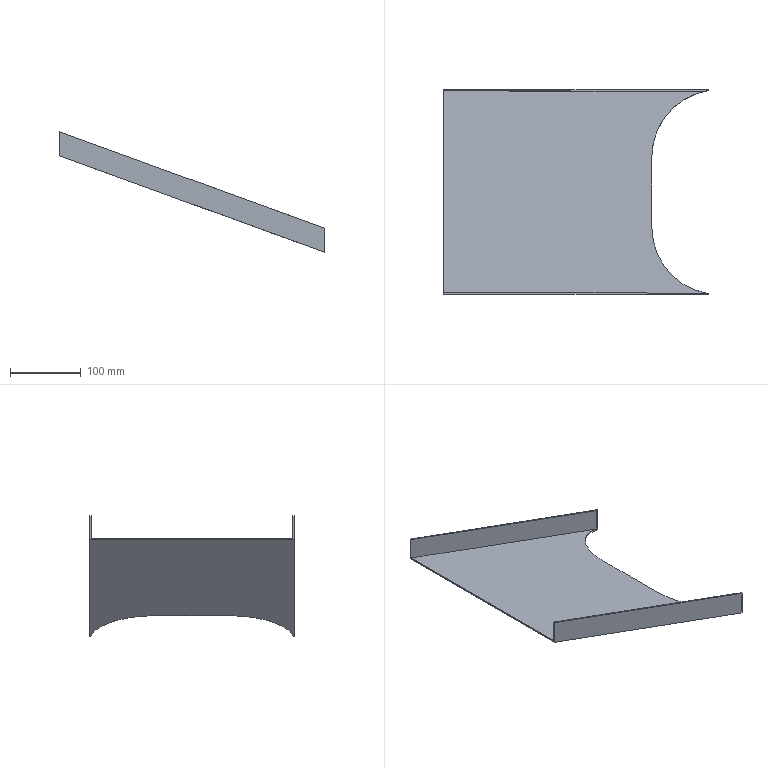Part | NX | features HB 2 | 1 solid | 14 faces | box 374.921 x 290 x 170.514 mm | volume 238011 mm3 | plane 12 | cylinder 2 | commonest cylinder face diameters 190 x2
STEP:
#1=CARTESIAN_POINT('',(630.,145.,-457.474));
#2=VERTEX_POINT('',#1);
#3=CARTESIAN_POINT('',(630.,143.808,-457.474));
#4=VERTEX_POINT('',#3);
#5=CARTESIAN_POINT('',(630.,203.921,-457.474));
#6=DIRECTION('',(0.,-1.,0.));
#7=VECTOR('',#6,1000.);
#8=LINE('',#5,#7);
#9=EDGE_CURVE('',#2,#4,#8,.T.);
#10=ORIENTED_EDGE('',*,*,#9,.T.);
#11=CARTESIAN_POINT('',(630.,143.808,-491.528));
#12=VERTEX_POINT('',#11);
#13=CARTESIAN_POINT('',(630.,143.808,-1480.5));
#14=DIRECTION('',(0.,0.,-1.));
#15=VECTOR('',#14,1000.);
#16=LINE('',#13,#15);
#17=EDGE_CURVE('',#4,#12,#16,.T.);
#18=ORIENTED_EDGE('',*,*,#17,.T.);
#19=CARTESIAN_POINT('',(630.,145.,-491.528));
#20=VERTEX_POINT('',#19);
#21=CARTESIAN_POINT('',(630.,98.921,-491.528));
#22=DIRECTION('',(0.,1.,0.));
#23=VECTOR('',#22,1000.);
#24=LINE('',#21,#23);
#25=EDGE_CURVE('',#12,#20,#24,.T.);
#26=ORIENTED_EDGE('',*,*,#25,.T.);
#27=CARTESIAN_POINT('',(630.,145.,-536.603));
#28=DIRECTION('',(0.,0.,1.));
#29=VECTOR('',#28,1000.);
#30=LINE('',#27,#29);
#31=EDGE_CURVE('',#20,#2,#30,.T.);
#32=ORIENTED_EDGE('',*,*,#31,.T.);
#33=EDGE_LOOP('',(#10,#18,#26,#32));
#34=FACE_BOUND('',#33,.T.);
#35=CARTESIAN_POINT('',(630.,0.,-678.5));
#36=DIRECTION('',(1.,0.,0.));
#37=DIRECTION('',(0.,0.,1.));
#38=AXIS2_PLACEMENT_3D('',#35,#36,#37);
#39=PLANE('',#38);
#40=ADVANCED_FACE('',(#34),#39,.T.);
#41=CARTESIAN_POINT('',(630.,-145.,-491.528));
#42=VERTEX_POINT('',#41);
#43=CARTESIAN_POINT('',(630.,-143.808,-491.528));
#44=VERTEX_POINT('',#43);
#45=CARTESIAN_POINT('',(630.,98.921,-491.528));
#46=DIRECTION('',(0.,1.,0.));
#47=VECTOR('',#46,1000.);
#48=LINE('',#45,#47);
#49=EDGE_CURVE('',#42,#44,#48,.T.);
#50=ORIENTED_EDGE('',*,*,#49,.T.);
#51=CARTESIAN_POINT('',(630.,-143.808,-457.474));
#52=VERTEX_POINT('',#51);
#53=CARTESIAN_POINT('',(630.,-143.808,-1480.5));
#54=DIRECTION('',(0.,0.,1.));
#55=VECTOR('',#54,1000.);
#56=LINE('',#53,#55);
#57=EDGE_CURVE('',#44,#52,#56,.T.);
#58=ORIENTED_EDGE('',*,*,#57,.T.);
#59=CARTESIAN_POINT('',(630.,-145.,-457.474));
#60=VERTEX_POINT('',#59);
#61=CARTESIAN_POINT('',(630.,-133.079,-457.474));
#62=DIRECTION('',(0.,-1.,0.));
#63=VECTOR('',#62,1000.);
#64=LINE('',#61,#63);
#65=EDGE_CURVE('',#52,#60,#64,.T.);
#66=ORIENTED_EDGE('',*,*,#65,.T.);
#67=CARTESIAN_POINT('',(630.,-145.,-2230.5));
#68=DIRECTION('',(0.,0.,-1.));
#69=VECTOR('',#68,1000.);
#70=LINE('',#67,#69);
#71=EDGE_CURVE('',#60,#42,#70,.T.);
#72=ORIENTED_EDGE('',*,*,#71,.T.);
#73=EDGE_LOOP('',(#50,#58,#66,#72));
#74=FACE_BOUND('',#73,.T.);
#75=CARTESIAN_POINT('',(630.,0.,-678.5));
#76=DIRECTION('',(1.,0.,0.));
#77=DIRECTION('',(0.,0.,1.));
#78=AXIS2_PLACEMENT_3D('',#75,#76,#77);
#79=PLANE('',#78);
#80=ADVANCED_FACE('',(#74),#79,.T.);
#81=CARTESIAN_POINT('',(625.609,-143.,-455.876));
#82=VERTEX_POINT('',#81);
#83=CARTESIAN_POINT('',(255.079,-143.,-321.014));
#84=VERTEX_POINT('',#83);
#85=CARTESIAN_POINT('',(1221.915,-143.,-672.914));
#86=DIRECTION('',(-0.9397,0.,0.342));
#87=VECTOR('',#86,1000.);
#88=LINE('',#85,#87);
#89=EDGE_CURVE('',#82,#84,#88,.T.);
#90=ORIENTED_EDGE('',*,*,#89,.F.);
#91=CARTESIAN_POINT('',(625.609,-143.,-487.801));
#92=VERTEX_POINT('',#91);
#93=CARTESIAN_POINT('',(625.609,-143.,-1480.5));
#94=DIRECTION('',(0.,0.,1.));
#95=VECTOR('',#94,1000.);
#96=LINE('',#93,#95);
#97=EDGE_CURVE('',#92,#82,#96,.T.);
#98=ORIENTED_EDGE('',*,*,#97,.F.);
#99=CARTESIAN_POINT('',(255.079,-143.,-352.939));
#100=VERTEX_POINT('',#99);
#101=CARTESIAN_POINT('',(1211.654,-143.,-701.104));
#102=DIRECTION('',(0.9397,0.,-0.342));
#103=VECTOR('',#102,1000.);
#104=LINE('',#101,#103);
#105=EDGE_CURVE('',#100,#92,#104,.T.);
#106=ORIENTED_EDGE('',*,*,#105,.F.);
#107=CARTESIAN_POINT('',(255.079,-143.,-160.));
#108=DIRECTION('',(0.,0.,-1.));
#109=VECTOR('',#108,1000.);
#110=LINE('',#107,#109);
#111=EDGE_CURVE('',#84,#100,#110,.T.);
#112=ORIENTED_EDGE('',*,*,#111,.F.);
#113=EDGE_LOOP('',(#90,#98,#106,#112));
#114=FACE_BOUND('',#113,.T.);
#115=CARTESIAN_POINT('',(655.,-143.,-2230.5));
#116=DIRECTION('',(0.,-1.,0.));
#117=DIRECTION('',(0.,0.,1.));
#118=AXIS2_PLACEMENT_3D('',#115,#116,#117);
#119=PLANE('',#118);
#120=ADVANCED_FACE('',(#114),#119,.F.);
#121=CARTESIAN_POINT('',(625.609,143.,-487.801));
#122=VERTEX_POINT('',#121);
#123=CARTESIAN_POINT('',(255.079,143.,-352.939));
#124=VERTEX_POINT('',#123);
#125=CARTESIAN_POINT('',(759.69,143.,-536.603));
#126=DIRECTION('',(-0.9397,0.,0.342));
#127=VECTOR('',#126,1000.);
#128=LINE('',#125,#127);
#129=EDGE_CURVE('',#122,#124,#128,.T.);
#130=ORIENTED_EDGE('',*,*,#129,.F.);
#131=CARTESIAN_POINT('',(625.609,143.,-455.876));
#132=VERTEX_POINT('',#131);
#133=CARTESIAN_POINT('',(625.609,143.,-1480.5));
#134=DIRECTION('',(0.,0.,1.));
#135=VECTOR('',#134,1000.);
#136=LINE('',#133,#135);
#137=EDGE_CURVE('',#122,#132,#136,.T.);
#138=ORIENTED_EDGE('',*,*,#137,.T.);
#139=CARTESIAN_POINT('',(255.079,143.,-321.014));
#140=VERTEX_POINT('',#139);
#141=CARTESIAN_POINT('',(769.951,143.,-508.412));
#142=DIRECTION('',(-0.9397,0.,0.342));
#143=VECTOR('',#142,1000.);
#144=LINE('',#141,#143);
#145=EDGE_CURVE('',#132,#140,#144,.T.);
#146=ORIENTED_EDGE('',*,*,#145,.T.);
#147=CARTESIAN_POINT('',(255.079,143.,-536.603));
#148=DIRECTION('',(0.,0.,1.));
#149=VECTOR('',#148,1000.);
#150=LINE('',#147,#149);
#151=EDGE_CURVE('',#124,#140,#150,.T.);
#152=ORIENTED_EDGE('',*,*,#151,.F.);
#153=EDGE_LOOP('',(#130,#138,#146,#152));
#154=FACE_BOUND('',#153,.T.);
#155=CARTESIAN_POINT('',(759.69,143.,-536.603));
#156=DIRECTION('',(0.,-1.,0.));
#157=DIRECTION('',(-0.08716,0.,0.9962));
#158=AXIS2_PLACEMENT_3D('',#155,#156,#157);
#159=PLANE('',#158);
#160=ADVANCED_FACE('',(#154),#159,.T.);
#161=CARTESIAN_POINT('',(645.,-50.,-462.934));
#162=DIRECTION('',(0.342,0.,0.9397));
#163=DIRECTION('',(-0.9397,0.,0.342));
#164=AXIS2_PLACEMENT_3D('',#161,#162,#163);
#165=ELLIPSE('',#164,101.097,95.);
#166=EDGE_CURVE('',#82,#52,#165,.T.);
#167=ORIENTED_EDGE('',*,*,#166,.F.);
#168=ORIENTED_EDGE('',*,*,#89,.T.);
#169=CARTESIAN_POINT('',(255.079,-145.,-321.014));
#170=VERTEX_POINT('',#169);
#171=CARTESIAN_POINT('',(255.079,-410.079,-321.014));
#172=DIRECTION('',(0.,-1.,0.));
#173=VECTOR('',#172,1000.);
#174=LINE('',#171,#173);
#175=EDGE_CURVE('',#84,#170,#174,.T.);
#176=ORIENTED_EDGE('',*,*,#175,.T.);
#177=CARTESIAN_POINT('',(1221.915,-145.,-672.914));
#178=DIRECTION('',(-0.9397,0.,0.342));
#179=VECTOR('',#178,1000.);
#180=LINE('',#177,#179);
#181=EDGE_CURVE('',#60,#170,#180,.T.);
#182=ORIENTED_EDGE('',*,*,#181,.F.);
#183=ORIENTED_EDGE('',*,*,#65,.F.);
#184=EDGE_LOOP('',(#167,#168,#176,#182,#183));
#185=FACE_BOUND('',#184,.T.);
#186=CARTESIAN_POINT('',(769.951,-133.079,-508.412));
#187=DIRECTION('',(-0.342,0.,-0.9397));
#188=DIRECTION('',(0.9397,0.,-0.342));
#189=AXIS2_PLACEMENT_3D('',#186,#187,#188);
#190=PLANE('',#189);
#191=ADVANCED_FACE('',(#185),#190,.F.);
#192=CARTESIAN_POINT('',(645.,50.,-462.934));
#193=DIRECTION('',(-0.342,0.,-0.9397));
#194=DIRECTION('',(-0.9397,0.,0.342));
#195=AXIS2_PLACEMENT_3D('',#192,#193,#194);
#196=ELLIPSE('',#195,101.097,95.);
#197=EDGE_CURVE('',#132,#4,#196,.T.);
#198=ORIENTED_EDGE('',*,*,#197,.T.);
#199=ORIENTED_EDGE('',*,*,#9,.F.);
#200=CARTESIAN_POINT('',(255.079,145.,-321.014));
#201=VERTEX_POINT('',#200);
#202=CARTESIAN_POINT('',(769.951,145.,-508.412));
#203=DIRECTION('',(-0.9397,0.,0.342));
#204=VECTOR('',#203,1000.);
#205=LINE('',#202,#204);
#206=EDGE_CURVE('',#2,#201,#205,.T.);
#207=ORIENTED_EDGE('',*,*,#206,.T.);
#208=CARTESIAN_POINT('',(255.079,-410.079,-321.014));
#209=DIRECTION('',(0.,-1.,0.));
#210=VECTOR('',#209,1000.);
#211=LINE('',#208,#210);
#212=EDGE_CURVE('',#201,#140,#211,.T.);
#213=ORIENTED_EDGE('',*,*,#212,.T.);
#214=ORIENTED_EDGE('',*,*,#145,.F.);
#215=EDGE_LOOP('',(#198,#199,#207,#213,#214));
#216=FACE_BOUND('',#215,.T.);
#217=CARTESIAN_POINT('',(769.951,203.921,-508.412));
#218=DIRECTION('',(-0.342,0.,-0.9397));
#219=DIRECTION('',(0.9397,0.,-0.342));
#220=AXIS2_PLACEMENT_3D('',#217,#218,#219);
#221=PLANE('',#220);
#222=ADVANCED_FACE('',(#216),#221,.F.);
#223=CARTESIAN_POINT('',(550.,50.,-460.282));
#224=VERTEX_POINT('',#223);
#225=CARTESIAN_POINT('',(550.,-50.,-460.282));
#226=VERTEX_POINT('',#225);
#227=CARTESIAN_POINT('',(550.,98.921,-460.282));
#228=DIRECTION('',(0.,-1.,0.));
#229=VECTOR('',#228,1000.);
#230=LINE('',#227,#229);
#231=EDGE_CURVE('',#224,#226,#230,.T.);
#232=ORIENTED_EDGE('',*,*,#231,.F.);
#233=CARTESIAN_POINT('',(645.,50.,-494.859));
#234=DIRECTION('',(0.342,0.,0.9397));
#235=DIRECTION('',(-0.9397,0.,0.342));
#236=AXIS2_PLACEMENT_3D('',#233,#234,#235);
#237=ELLIPSE('',#236,101.097,95.);
#238=EDGE_CURVE('',#122,#224,#237,.T.);
#239=ORIENTED_EDGE('',*,*,#238,.F.);
#240=ORIENTED_EDGE('',*,*,#129,.T.);
#241=CARTESIAN_POINT('',(255.079,-410.079,-352.939));
#242=DIRECTION('',(0.,1.,0.));
#243=VECTOR('',#242,1000.);
#244=LINE('',#241,#243);
#245=EDGE_CURVE('',#100,#124,#244,.T.);
#246=ORIENTED_EDGE('',*,*,#245,.F.);
#247=ORIENTED_EDGE('',*,*,#105,.T.);
#248=CARTESIAN_POINT('',(645.,-50.,-494.859));
#249=DIRECTION('',(0.342,0.,0.9397));
#250=DIRECTION('',(-0.9397,0.,0.342));
#251=AXIS2_PLACEMENT_3D('',#248,#249,#250);
#252=ELLIPSE('',#251,101.097,95.);
#253=EDGE_CURVE('',#226,#92,#252,.T.);
#254=ORIENTED_EDGE('',*,*,#253,.F.);
#255=EDGE_LOOP('',(#232,#239,#240,#246,#247,#254));
#256=FACE_BOUND('',#255,.T.);
#257=CARTESIAN_POINT('',(759.69,98.921,-536.603));
#258=DIRECTION('',(0.342,0.,0.9397));
#259=DIRECTION('',(0.,-1.,0.));
#260=AXIS2_PLACEMENT_3D('',#257,#258,#259);
#261=PLANE('',#260);
#262=ADVANCED_FACE('',(#256),#261,.T.);
#263=CARTESIAN_POINT('',(550.,50.,-462.41));
#264=VERTEX_POINT('',#263);
#265=CARTESIAN_POINT('',(645.,50.,-496.987));
#266=DIRECTION('',(-0.342,0.,-0.9397));
#267=DIRECTION('',(-0.9397,0.,0.342));
#268=AXIS2_PLACEMENT_3D('',#265,#266,#267);
#269=ELLIPSE('',#268,101.097,95.);
#270=EDGE_CURVE('',#264,#12,#269,.T.);
#271=ORIENTED_EDGE('',*,*,#270,.F.);
#272=CARTESIAN_POINT('',(550.,-50.,-462.41));
#273=VERTEX_POINT('',#272);
#274=CARTESIAN_POINT('',(550.,98.921,-462.41));
#275=DIRECTION('',(0.,1.,0.));
#276=VECTOR('',#275,1000.);
#277=LINE('',#274,#276);
#278=EDGE_CURVE('',#273,#264,#277,.T.);
#279=ORIENTED_EDGE('',*,*,#278,.F.);
#280=CARTESIAN_POINT('',(645.,-50.,-496.987));
#281=DIRECTION('',(0.342,0.,0.9397));
#282=DIRECTION('',(-0.9397,0.,0.342));
#283=AXIS2_PLACEMENT_3D('',#280,#281,#282);
#284=ELLIPSE('',#283,101.097,95.);
#285=EDGE_CURVE('',#273,#44,#284,.T.);
#286=ORIENTED_EDGE('',*,*,#285,.T.);
#287=ORIENTED_EDGE('',*,*,#49,.F.);
#288=CARTESIAN_POINT('',(255.079,-145.,-355.068));
#289=VERTEX_POINT('',#288);
#290=CARTESIAN_POINT('',(759.006,-145.,-538.482));
#291=DIRECTION('',(-0.9397,0.,0.342));
#292=VECTOR('',#291,1000.);
#293=LINE('',#290,#292);
#294=EDGE_CURVE('',#42,#289,#293,.T.);
#295=ORIENTED_EDGE('',*,*,#294,.T.);
#296=CARTESIAN_POINT('',(255.079,145.,-355.068));
#297=VERTEX_POINT('',#296);
#298=CARTESIAN_POINT('',(255.079,-410.079,-355.068));
#299=DIRECTION('',(0.,1.,0.));
#300=VECTOR('',#299,1000.);
#301=LINE('',#298,#300);
#302=EDGE_CURVE('',#289,#297,#301,.T.);
#303=ORIENTED_EDGE('',*,*,#302,.T.);
#304=CARTESIAN_POINT('',(759.006,145.,-538.482));
#305=DIRECTION('',(0.9397,0.,-0.342));
#306=VECTOR('',#305,1000.);
#307=LINE('',#304,#306);
#308=EDGE_CURVE('',#297,#20,#307,.T.);
#309=ORIENTED_EDGE('',*,*,#308,.T.);
#310=ORIENTED_EDGE('',*,*,#25,.F.);
#311=EDGE_LOOP('',(#271,#279,#286,#287,#295,#303,#309,#310));
#312=FACE_BOUND('',#311,.T.);
#313=CARTESIAN_POINT('',(759.006,98.921,-538.482));
#314=DIRECTION('',(0.342,0.,0.9397));
#315=DIRECTION('',(0.,-1.,0.));
#316=AXIS2_PLACEMENT_3D('',#313,#314,#315);
#317=PLANE('',#316);
#318=ADVANCED_FACE('',(#312),#317,.F.);
#319=ORIENTED_EDGE('',*,*,#31,.F.);
#320=ORIENTED_EDGE('',*,*,#308,.F.);
#321=CARTESIAN_POINT('',(255.079,145.,-536.603));
#322=DIRECTION('',(0.,0.,1.));
#323=VECTOR('',#322,1000.);
#324=LINE('',#321,#323);
#325=EDGE_CURVE('',#297,#201,#324,.T.);
#326=ORIENTED_EDGE('',*,*,#325,.T.);
#327=ORIENTED_EDGE('',*,*,#206,.F.);
#328=EDGE_LOOP('',(#319,#320,#326,#327));
#329=FACE_BOUND('',#328,.T.);
#330=CARTESIAN_POINT('',(759.69,145.,-536.603));
#331=DIRECTION('',(0.,-1.,0.));
#332=DIRECTION('',(0.08716,0.,-0.9962));
#333=AXIS2_PLACEMENT_3D('',#330,#331,#332);
#334=PLANE('',#333);
#335=ADVANCED_FACE('',(#329),#334,.F.);
#336=ORIENTED_EDGE('',*,*,#71,.F.);
#337=ORIENTED_EDGE('',*,*,#181,.T.);
#338=CARTESIAN_POINT('',(255.079,-145.,-160.));
#339=DIRECTION('',(0.,0.,-1.));
#340=VECTOR('',#339,1000.);
#341=LINE('',#338,#340);
#342=EDGE_CURVE('',#170,#289,#341,.T.);
#343=ORIENTED_EDGE('',*,*,#342,.T.);
#344=ORIENTED_EDGE('',*,*,#294,.F.);
#345=EDGE_LOOP('',(#336,#337,#343,#344));
#346=FACE_BOUND('',#345,.T.);
#347=CARTESIAN_POINT('',(655.,-145.,-2230.5));
#348=DIRECTION('',(0.,-1.,0.));
#349=DIRECTION('',(0.,0.,1.));
#350=AXIS2_PLACEMENT_3D('',#347,#348,#349);
#351=PLANE('',#350);
#352=ADVANCED_FACE('',(#346),#351,.T.);
#353=ORIENTED_EDGE('',*,*,#302,.F.);
#354=ORIENTED_EDGE('',*,*,#342,.F.);
#355=ORIENTED_EDGE('',*,*,#175,.F.);
#356=ORIENTED_EDGE('',*,*,#111,.T.);
#357=ORIENTED_EDGE('',*,*,#245,.T.);
#358=ORIENTED_EDGE('',*,*,#151,.T.);
#359=ORIENTED_EDGE('',*,*,#212,.F.);
#360=ORIENTED_EDGE('',*,*,#325,.F.);
#361=EDGE_LOOP('',(#353,#354,#355,#356,#357,#358,#359,#360));
#362=FACE_BOUND('',#361,.T.);
#363=CARTESIAN_POINT('',(255.079,-410.079,-160.));
#364=DIRECTION('',(-1.,0.,0.));
#365=DIRECTION('',(0.,0.,-1.));
#366=AXIS2_PLACEMENT_3D('',#363,#364,#365);
#367=PLANE('',#366);
#368=ADVANCED_FACE('',(#362),#367,.T.);
#369=ORIENTED_EDGE('',*,*,#231,.T.);
#370=CARTESIAN_POINT('',(550.,-50.,-1480.5));
#371=DIRECTION('',(0.,0.,1.));
#372=VECTOR('',#371,1000.);
#373=LINE('',#370,#372);
#374=EDGE_CURVE('',#273,#226,#373,.T.);
#375=ORIENTED_EDGE('',*,*,#374,.F.);
#376=ORIENTED_EDGE('',*,*,#278,.T.);
#377=CARTESIAN_POINT('',(550.,50.,-1480.5));
#378=DIRECTION('',(0.,0.,1.));
#379=VECTOR('',#378,1000.);
#380=LINE('',#377,#379);
#381=EDGE_CURVE('',#264,#224,#380,.T.);
#382=ORIENTED_EDGE('',*,*,#381,.T.);
#383=EDGE_LOOP('',(#369,#375,#376,#382));
#384=FACE_BOUND('',#383,.T.);
#385=CARTESIAN_POINT('',(550.,-50.,-1480.5));
#386=DIRECTION('',(1.,0.,0.));
#387=DIRECTION('',(0.,0.,1.));
#388=AXIS2_PLACEMENT_3D('',#385,#386,#387);
#389=PLANE('',#388);
#390=ADVANCED_FACE('',(#384),#389,.T.);
#391=ORIENTED_EDGE('',*,*,#238,.T.);
#392=ORIENTED_EDGE('',*,*,#381,.F.);
#393=ORIENTED_EDGE('',*,*,#270,.T.);
#394=ORIENTED_EDGE('',*,*,#17,.F.);
#395=ORIENTED_EDGE('',*,*,#197,.F.);
#396=ORIENTED_EDGE('',*,*,#137,.F.);
#397=EDGE_LOOP('',(#391,#392,#393,#394,#395,#396));
#398=FACE_BOUND('',#397,.T.);
#399=CARTESIAN_POINT('',(645.,50.,-1480.5));
#400=DIRECTION('',(0.,0.,1.));
#401=DIRECTION('',(-1.,0.,0.));
#402=AXIS2_PLACEMENT_3D('',#399,#400,#401);
#403=CYLINDRICAL_SURFACE('',#402,95.);
#404=ADVANCED_FACE('',(#398),#403,.F.);
#405=ORIENTED_EDGE('',*,*,#253,.T.);
#406=ORIENTED_EDGE('',*,*,#97,.T.);
#407=ORIENTED_EDGE('',*,*,#166,.T.);
#408=ORIENTED_EDGE('',*,*,#57,.F.);
#409=ORIENTED_EDGE('',*,*,#285,.F.);
#410=ORIENTED_EDGE('',*,*,#374,.T.);
#411=EDGE_LOOP('',(#405,#406,#407,#408,#409,#410));
#412=FACE_BOUND('',#411,.T.);
#413=CARTESIAN_POINT('',(645.,-50.,-1480.5));
#414=DIRECTION('',(0.,0.,1.));
#415=DIRECTION('',(-1.,0.,0.));
#416=AXIS2_PLACEMENT_3D('',#413,#414,#415);
#417=CYLINDRICAL_SURFACE('',#416,95.);
#418=ADVANCED_FACE('',(#412),#417,.F.);
#419=CLOSED_SHELL('',(#40,#80,#120,#160,#191,#222,#262,#318,#335,#352,#368,#390,#404,#418));
#420=MANIFOLD_SOLID_BREP('',#419);
#421=(LENGTH_UNIT()NAMED_UNIT(*)SI_UNIT(.MILLI.,.METRE.));
#422=UNCERTAINTY_MEASURE_WITH_UNIT(LENGTH_MEASURE(0.00001),#421,'','');
#423=(NAMED_UNIT(*)PLANE_ANGLE_UNIT()SI_UNIT($,.RADIAN.));
#424=(NAMED_UNIT(*)SI_UNIT($,.STERADIAN.)SOLID_ANGLE_UNIT());
#425=(GEOMETRIC_REPRESENTATION_CONTEXT(3)GLOBAL_UNCERTAINTY_ASSIGNED_CONTEXT((#422))GLOBAL_UNIT_ASSIGNED_CONTEXT((#421,#423,#424))REPRESENTATION_CONTEXT('',''));
#426=ADVANCED_BREP_SHAPE_REPRESENTATION('',(#420),#425);